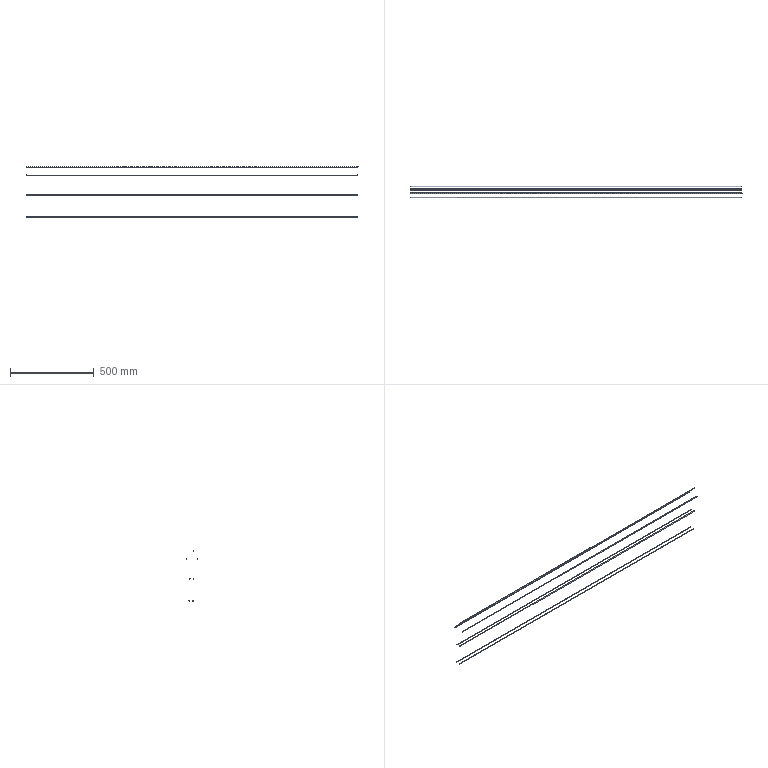Part | SolidWorks | features BaseBody 7 | 7 solids | 28 faces | box 1977 x 68.151 x 299.907 mm | volume 173588 mm3 | cylinder 14 | plane 14 | commonest cylinder face diameters 4 x14
STEP:
#1=CARTESIAN_POINT('',(-25.106,43.452,97.628));
#2=VERTEX_POINT('',#1);
#3=CARTESIAN_POINT('',(-25.106,39.452,97.628));
#4=VERTEX_POINT('',#3);
#5=CARTESIAN_POINT('',(-25.106,43.452,97.628));
#6=CARTESIAN_POINT('',(-24.91,43.452,101.628));
#7=CARTESIAN_POINT('',(-24.91,39.452,101.628));
#8=CARTESIAN_POINT('',(-25.106,39.452,97.628));
#9=(BOUNDED_CURVE()B_SPLINE_CURVE(3,(#5,#6,#7,#8),.UNSPECIFIED.,.F.,.F.)B_SPLINE_CURVE_WITH_KNOTS((4,4),(1.571,4.712),.UNSPECIFIED.)CURVE()GEOMETRIC_REPRESENTATION_ITEM()RATIONAL_B_SPLINE_CURVE((1.,0.3333,0.3333,1.))REPRESENTATION_ITEM(''));
#10=EDGE_CURVE('',#2,#4,#9,.T.);
#11=ORIENTED_EDGE('',*,*,#10,.F.);
#12=CARTESIAN_POINT('',(-2000.,43.452,97.628));
#13=VERTEX_POINT('',#12);
#14=CARTESIAN_POINT('',(-13.158,43.452,97.628));
#15=DIRECTION('',(-1.,0.,0.));
#16=VECTOR('',#15,1000.);
#17=LINE('',#14,#16);
#18=EDGE_CURVE('',#2,#13,#17,.T.);
#19=ORIENTED_EDGE('',*,*,#18,.T.);
#20=CARTESIAN_POINT('',(-2000.,39.452,97.628));
#21=VERTEX_POINT('',#20);
#22=CARTESIAN_POINT('',(-2000.,41.452,97.628));
#23=DIRECTION('',(-1.,0.,0.));
#24=DIRECTION('',(0.,-1.,0.));
#25=AXIS2_PLACEMENT_3D('',#22,#23,#24);
#26=CIRCLE('',#25,2.);
#27=EDGE_CURVE('',#21,#13,#26,.T.);
#28=ORIENTED_EDGE('',*,*,#27,.F.);
#29=CARTESIAN_POINT('',(-13.158,39.452,97.628));
#30=DIRECTION('',(-1.,0.,0.));
#31=VECTOR('',#30,1000.);
#32=LINE('',#29,#31);
#33=EDGE_CURVE('',#4,#21,#32,.T.);
#34=ORIENTED_EDGE('',*,*,#33,.F.);
#35=EDGE_LOOP('',(#11,#19,#28,#34));
#36=FACE_OUTER_BOUND('',#35,.T.);
#37=CARTESIAN_POINT('',(-13.158,41.452,97.628));
#38=DIRECTION('',(-1.,0.,0.));
#39=DIRECTION('',(0.,-1.,0.));
#40=AXIS2_PLACEMENT_3D('',#37,#38,#39);
#41=CYLINDRICAL_SURFACE('',#40,2.);
#42=ADVANCED_FACE('',(#36),#41,.T.);
#43=ORIENTED_EDGE('',*,*,#18,.F.);
#44=CARTESIAN_POINT('',(-25.106,39.452,97.628));
#45=CARTESIAN_POINT('',(-25.302,39.452,93.628));
#46=CARTESIAN_POINT('',(-25.302,43.452,93.628));
#47=CARTESIAN_POINT('',(-25.106,43.452,97.628));
#48=(BOUNDED_CURVE()B_SPLINE_CURVE(3,(#44,#45,#46,#47),.UNSPECIFIED.,.F.,.F.)B_SPLINE_CURVE_WITH_KNOTS((4,4),(4.712,7.854),.UNSPECIFIED.)CURVE()GEOMETRIC_REPRESENTATION_ITEM()RATIONAL_B_SPLINE_CURVE((1.,0.3333,0.3333,1.))REPRESENTATION_ITEM(''));
#49=EDGE_CURVE('',#4,#2,#48,.T.);
#50=ORIENTED_EDGE('',*,*,#49,.F.);
#51=ORIENTED_EDGE('',*,*,#33,.T.);
#52=CARTESIAN_POINT('',(-2000.,41.452,97.628));
#53=DIRECTION('',(-1.,0.,0.));
#54=DIRECTION('',(0.,-1.,0.));
#55=AXIS2_PLACEMENT_3D('',#52,#53,#54);
#56=CIRCLE('',#55,2.);
#57=EDGE_CURVE('',#13,#21,#56,.T.);
#58=ORIENTED_EDGE('',*,*,#57,.F.);
#59=EDGE_LOOP('',(#43,#50,#51,#58));
#60=FACE_OUTER_BOUND('',#59,.T.);
#61=CARTESIAN_POINT('',(-13.158,41.452,97.628));
#62=DIRECTION('',(-1.,0.,0.));
#63=DIRECTION('',(0.,-1.,0.));
#64=AXIS2_PLACEMENT_3D('',#61,#62,#63);
#65=CYLINDRICAL_SURFACE('',#64,2.);
#66=ADVANCED_FACE('',(#60),#65,.T.);
#67=ORIENTED_EDGE('',*,*,#49,.T.);
#68=ORIENTED_EDGE('',*,*,#10,.T.);
#69=EDGE_LOOP('',(#67,#68));
#70=FACE_OUTER_BOUND('',#69,.T.);
#71=CARTESIAN_POINT('',(-25.205,39.428,95.604));
#72=DIRECTION('',(-0.9988,0.,0.04903));
#73=DIRECTION('',(0.04903,0.,0.9988));
#74=AXIS2_PLACEMENT_3D('',#71,#72,#73);
#75=PLANE('',#74);
#76=ADVANCED_FACE('',(#70),#75,.F.);
#77=ORIENTED_EDGE('',*,*,#27,.T.);
#78=ORIENTED_EDGE('',*,*,#57,.T.);
#79=EDGE_LOOP('',(#77,#78));
#80=FACE_OUTER_BOUND('',#79,.T.);
#81=CARTESIAN_POINT('',(-2000.,39.428,99.652));
#82=DIRECTION('',(1.,0.,0.));
#83=DIRECTION('',(0.,0.,-1.));
#84=AXIS2_PLACEMENT_3D('',#81,#82,#83);
#85=PLANE('',#84);
#86=ADVANCED_FACE('',(#80),#85,.F.);
#87=CLOSED_SHELL('',(#42,#66,#76,#86));
#88=MANIFOLD_SOLID_BREP('',#87);
#89=CARTESIAN_POINT('',(-25.106,-20.7,97.628));
#90=VERTEX_POINT('',#89);
#91=CARTESIAN_POINT('',(-25.106,-24.7,97.628));
#92=VERTEX_POINT('',#91);
#93=CARTESIAN_POINT('',(-25.106,-20.7,97.628));
#94=CARTESIAN_POINT('',(-24.91,-20.7,101.628));
#95=CARTESIAN_POINT('',(-24.91,-24.7,101.628));
#96=CARTESIAN_POINT('',(-25.106,-24.7,97.628));
#97=(BOUNDED_CURVE()B_SPLINE_CURVE(3,(#93,#94,#95,#96),.UNSPECIFIED.,.F.,.F.)B_SPLINE_CURVE_WITH_KNOTS((4,4),(1.571,4.712),.UNSPECIFIED.)CURVE()GEOMETRIC_REPRESENTATION_ITEM()RATIONAL_B_SPLINE_CURVE((1.,0.3333,0.3333,1.))REPRESENTATION_ITEM(''));
#98=EDGE_CURVE('',#90,#92,#97,.T.);
#99=ORIENTED_EDGE('',*,*,#98,.F.);
#100=CARTESIAN_POINT('',(-2000.,-20.7,97.628));
#101=VERTEX_POINT('',#100);
#102=CARTESIAN_POINT('',(-13.158,-20.7,97.628));
#103=DIRECTION('',(-1.,0.,0.));
#104=VECTOR('',#103,1000.);
#105=LINE('',#102,#104);
#106=EDGE_CURVE('',#90,#101,#105,.T.);
#107=ORIENTED_EDGE('',*,*,#106,.T.);
#108=CARTESIAN_POINT('',(-2000.,-24.7,97.628));
#109=VERTEX_POINT('',#108);
#110=CARTESIAN_POINT('',(-2000.,-22.7,97.628));
#111=DIRECTION('',(-1.,0.,0.));
#112=DIRECTION('',(0.,-1.,0.));
#113=AXIS2_PLACEMENT_3D('',#110,#111,#112);
#114=CIRCLE('',#113,2.);
#115=EDGE_CURVE('',#109,#101,#114,.T.);
#116=ORIENTED_EDGE('',*,*,#115,.F.);
#117=CARTESIAN_POINT('',(-13.158,-24.7,97.628));
#118=DIRECTION('',(-1.,0.,0.));
#119=VECTOR('',#118,1000.);
#120=LINE('',#117,#119);
#121=EDGE_CURVE('',#92,#109,#120,.T.);
#122=ORIENTED_EDGE('',*,*,#121,.F.);
#123=EDGE_LOOP('',(#99,#107,#116,#122));
#124=FACE_OUTER_BOUND('',#123,.T.);
#125=CARTESIAN_POINT('',(-13.158,-22.7,97.628));
#126=DIRECTION('',(-1.,0.,0.));
#127=DIRECTION('',(0.,-1.,0.));
#128=AXIS2_PLACEMENT_3D('',#125,#126,#127);
#129=CYLINDRICAL_SURFACE('',#128,2.);
#130=ADVANCED_FACE('',(#124),#129,.T.);
#131=ORIENTED_EDGE('',*,*,#106,.F.);
#132=CARTESIAN_POINT('',(-25.106,-24.7,97.628));
#133=CARTESIAN_POINT('',(-25.302,-24.7,93.628));
#134=CARTESIAN_POINT('',(-25.302,-20.7,93.628));
#135=CARTESIAN_POINT('',(-25.106,-20.7,97.628));
#136=(BOUNDED_CURVE()B_SPLINE_CURVE(3,(#132,#133,#134,#135),.UNSPECIFIED.,.F.,.F.)B_SPLINE_CURVE_WITH_KNOTS((4,4),(4.712,7.854),.UNSPECIFIED.)CURVE()GEOMETRIC_REPRESENTATION_ITEM()RATIONAL_B_SPLINE_CURVE((1.,0.3333,0.3333,1.))REPRESENTATION_ITEM(''));
#137=EDGE_CURVE('',#92,#90,#136,.T.);
#138=ORIENTED_EDGE('',*,*,#137,.F.);
#139=ORIENTED_EDGE('',*,*,#121,.T.);
#140=CARTESIAN_POINT('',(-2000.,-22.7,97.628));
#141=DIRECTION('',(-1.,0.,0.));
#142=DIRECTION('',(0.,-1.,0.));
#143=AXIS2_PLACEMENT_3D('',#140,#141,#142);
#144=CIRCLE('',#143,2.);
#145=EDGE_CURVE('',#101,#109,#144,.T.);
#146=ORIENTED_EDGE('',*,*,#145,.F.);
#147=EDGE_LOOP('',(#131,#138,#139,#146));
#148=FACE_OUTER_BOUND('',#147,.T.);
#149=CARTESIAN_POINT('',(-13.158,-22.7,97.628));
#150=DIRECTION('',(-1.,0.,0.));
#151=DIRECTION('',(0.,-1.,0.));
#152=AXIS2_PLACEMENT_3D('',#149,#150,#151);
#153=CYLINDRICAL_SURFACE('',#152,2.);
#154=ADVANCED_FACE('',(#148),#153,.T.);
#155=ORIENTED_EDGE('',*,*,#137,.T.);
#156=ORIENTED_EDGE('',*,*,#98,.T.);
#157=EDGE_LOOP('',(#155,#156));
#158=FACE_OUTER_BOUND('',#157,.T.);
#159=CARTESIAN_POINT('',(-25.205,-24.724,95.604));
#160=DIRECTION('',(-0.9988,0.,0.04903));
#161=DIRECTION('',(0.04903,0.,0.9988));
#162=AXIS2_PLACEMENT_3D('',#159,#160,#161);
#163=PLANE('',#162);
#164=ADVANCED_FACE('',(#158),#163,.F.);
#165=ORIENTED_EDGE('',*,*,#115,.T.);
#166=ORIENTED_EDGE('',*,*,#145,.T.);
#167=EDGE_LOOP('',(#165,#166));
#168=FACE_OUTER_BOUND('',#167,.T.);
#169=CARTESIAN_POINT('',(-2000.,-24.724,99.652));
#170=DIRECTION('',(1.,0.,0.));
#171=DIRECTION('',(0.,0.,-1.));
#172=AXIS2_PLACEMENT_3D('',#169,#170,#171);
#173=PLANE('',#172);
#174=ADVANCED_FACE('',(#168),#173,.F.);
#175=CLOSED_SHELL('',(#130,#154,#164,#174));
#176=MANIFOLD_SOLID_BREP('',#175);
#177=CARTESIAN_POINT('',(-28.322,27.021,-151.964));
#178=VERTEX_POINT('',#177);
#179=CARTESIAN_POINT('',(-28.322,27.021,-147.964));
#180=VERTEX_POINT('',#179);
#181=CARTESIAN_POINT('',(-28.322,27.021,-149.964));
#182=DIRECTION('',(1.,0.,0.));
#183=DIRECTION('',(0.,0.,1.));
#184=AXIS2_PLACEMENT_3D('',#181,#182,#183);
#185=CIRCLE('',#184,2.);
#186=EDGE_CURVE('',#178,#180,#185,.T.);
#187=ORIENTED_EDGE('',*,*,#186,.F.);
#188=CARTESIAN_POINT('',(-2000.,27.021,-151.964));
#189=VERTEX_POINT('',#188);
#190=CARTESIAN_POINT('',(-28.322,27.021,-151.964));
#191=DIRECTION('',(-1.,0.,0.));
#192=VECTOR('',#191,1000.);
#193=LINE('',#190,#192);
#194=EDGE_CURVE('',#178,#189,#193,.T.);
#195=ORIENTED_EDGE('',*,*,#194,.T.);
#196=CARTESIAN_POINT('',(-2000.,27.021,-147.964));
#197=VERTEX_POINT('',#196);
#198=CARTESIAN_POINT('',(-2000.,27.021,-149.964));
#199=DIRECTION('',(-1.,0.,0.));
#200=DIRECTION('',(0.,0.,1.));
#201=AXIS2_PLACEMENT_3D('',#198,#199,#200);
#202=CIRCLE('',#201,2.);
#203=EDGE_CURVE('',#197,#189,#202,.T.);
#204=ORIENTED_EDGE('',*,*,#203,.F.);
#205=CARTESIAN_POINT('',(-28.322,27.021,-147.964));
#206=DIRECTION('',(-1.,0.,0.));
#207=VECTOR('',#206,1000.);
#208=LINE('',#205,#207);
#209=EDGE_CURVE('',#180,#197,#208,.T.);
#210=ORIENTED_EDGE('',*,*,#209,.F.);
#211=EDGE_LOOP('',(#187,#195,#204,#210));
#212=FACE_OUTER_BOUND('',#211,.T.);
#213=CARTESIAN_POINT('',(-28.322,27.021,-149.964));
#214=DIRECTION('',(-1.,0.,0.));
#215=DIRECTION('',(0.,0.,1.));
#216=AXIS2_PLACEMENT_3D('',#213,#214,#215);
#217=CYLINDRICAL_SURFACE('',#216,2.);
#218=ADVANCED_FACE('',(#212),#217,.T.);
#219=ORIENTED_EDGE('',*,*,#194,.F.);
#220=CARTESIAN_POINT('',(-28.322,27.021,-149.964));
#221=DIRECTION('',(1.,0.,0.));
#222=DIRECTION('',(0.,0.,1.));
#223=AXIS2_PLACEMENT_3D('',#220,#221,#222);
#224=CIRCLE('',#223,2.);
#225=EDGE_CURVE('',#180,#178,#224,.T.);
#226=ORIENTED_EDGE('',*,*,#225,.F.);
#227=ORIENTED_EDGE('',*,*,#209,.T.);
#228=CARTESIAN_POINT('',(-2000.,27.021,-149.964));
#229=DIRECTION('',(-1.,0.,0.));
#230=DIRECTION('',(0.,0.,1.));
#231=AXIS2_PLACEMENT_3D('',#228,#229,#230);
#232=CIRCLE('',#231,2.);
#233=EDGE_CURVE('',#189,#197,#232,.T.);
#234=ORIENTED_EDGE('',*,*,#233,.F.);
#235=EDGE_LOOP('',(#219,#226,#227,#234));
#236=FACE_OUTER_BOUND('',#235,.T.);
#237=CARTESIAN_POINT('',(-28.322,27.021,-149.964));
#238=DIRECTION('',(-1.,0.,0.));
#239=DIRECTION('',(0.,0.,1.));
#240=AXIS2_PLACEMENT_3D('',#237,#238,#239);
#241=CYLINDRICAL_SURFACE('',#240,2.);
#242=ADVANCED_FACE('',(#236),#241,.T.);
#243=ORIENTED_EDGE('',*,*,#225,.T.);
#244=ORIENTED_EDGE('',*,*,#186,.T.);
#245=EDGE_LOOP('',(#243,#244));
#246=FACE_OUTER_BOUND('',#245,.T.);
#247=CARTESIAN_POINT('',(-28.322,24.997,-151.988));
#248=DIRECTION('',(-1.,0.,0.));
#249=DIRECTION('',(0.,0.,1.));
#250=AXIS2_PLACEMENT_3D('',#247,#248,#249);
#251=PLANE('',#250);
#252=ADVANCED_FACE('',(#246),#251,.F.);
#253=ORIENTED_EDGE('',*,*,#203,.T.);
#254=ORIENTED_EDGE('',*,*,#233,.T.);
#255=EDGE_LOOP('',(#253,#254));
#256=FACE_OUTER_BOUND('',#255,.T.);
#257=CARTESIAN_POINT('',(-2000.,24.997,-147.94));
#258=DIRECTION('',(1.,0.,0.));
#259=DIRECTION('',(0.,0.,-1.));
#260=AXIS2_PLACEMENT_3D('',#257,#258,#259);
#261=PLANE('',#260);
#262=ADVANCED_FACE('',(#256),#261,.F.);
#263=CLOSED_SHELL('',(#218,#242,#252,#262));
#264=MANIFOLD_SOLID_BREP('',#263);
#265=CARTESIAN_POINT('',(-28.322,3.953,-152.971));
#266=VERTEX_POINT('',#265);
#267=CARTESIAN_POINT('',(-28.322,3.953,-148.971));
#268=VERTEX_POINT('',#267);
#269=CARTESIAN_POINT('',(-28.322,3.953,-150.971));
#270=DIRECTION('',(1.,0.,0.));
#271=DIRECTION('',(0.,0.,1.));
#272=AXIS2_PLACEMENT_3D('',#269,#270,#271);
#273=CIRCLE('',#272,2.);
#274=EDGE_CURVE('',#266,#268,#273,.T.);
#275=ORIENTED_EDGE('',*,*,#274,.F.);
#276=CARTESIAN_POINT('',(-2000.,3.953,-152.971));
#277=VERTEX_POINT('',#276);
#278=CARTESIAN_POINT('',(-28.322,3.953,-152.971));
#279=DIRECTION('',(-1.,0.,0.));
#280=VECTOR('',#279,1000.);
#281=LINE('',#278,#280);
#282=EDGE_CURVE('',#266,#277,#281,.T.);
#283=ORIENTED_EDGE('',*,*,#282,.T.);
#284=CARTESIAN_POINT('',(-2000.,3.953,-148.971));
#285=VERTEX_POINT('',#284);
#286=CARTESIAN_POINT('',(-2000.,3.953,-150.971));
#287=DIRECTION('',(-1.,0.,0.));
#288=DIRECTION('',(0.,0.,1.));
#289=AXIS2_PLACEMENT_3D('',#286,#287,#288);
#290=CIRCLE('',#289,2.);
#291=EDGE_CURVE('',#285,#277,#290,.T.);
#292=ORIENTED_EDGE('',*,*,#291,.F.);
#293=CARTESIAN_POINT('',(-28.322,3.953,-148.971));
#294=DIRECTION('',(-1.,0.,0.));
#295=VECTOR('',#294,1000.);
#296=LINE('',#293,#295);
#297=EDGE_CURVE('',#268,#285,#296,.T.);
#298=ORIENTED_EDGE('',*,*,#297,.F.);
#299=EDGE_LOOP('',(#275,#283,#292,#298));
#300=FACE_OUTER_BOUND('',#299,.T.);
#301=CARTESIAN_POINT('',(-28.322,3.953,-150.971));
#302=DIRECTION('',(-1.,0.,0.));
#303=DIRECTION('',(0.,0.,1.));
#304=AXIS2_PLACEMENT_3D('',#301,#302,#303);
#305=CYLINDRICAL_SURFACE('',#304,2.);
#306=ADVANCED_FACE('',(#300),#305,.T.);
#307=ORIENTED_EDGE('',*,*,#282,.F.);
#308=CARTESIAN_POINT('',(-28.322,3.953,-150.971));
#309=DIRECTION('',(1.,0.,0.));
#310=DIRECTION('',(0.,0.,1.));
#311=AXIS2_PLACEMENT_3D('',#308,#309,#310);
#312=CIRCLE('',#311,2.);
#313=EDGE_CURVE('',#268,#266,#312,.T.);
#314=ORIENTED_EDGE('',*,*,#313,.F.);
#315=ORIENTED_EDGE('',*,*,#297,.T.);
#316=CARTESIAN_POINT('',(-2000.,3.953,-150.971));
#317=DIRECTION('',(-1.,0.,0.));
#318=DIRECTION('',(0.,0.,1.));
#319=AXIS2_PLACEMENT_3D('',#316,#317,#318);
#320=CIRCLE('',#319,2.);
#321=EDGE_CURVE('',#277,#285,#320,.T.);
#322=ORIENTED_EDGE('',*,*,#321,.F.);
#323=EDGE_LOOP('',(#307,#314,#315,#322));
#324=FACE_OUTER_BOUND('',#323,.T.);
#325=CARTESIAN_POINT('',(-28.322,3.953,-150.971));
#326=DIRECTION('',(-1.,0.,0.));
#327=DIRECTION('',(0.,0.,1.));
#328=AXIS2_PLACEMENT_3D('',#325,#326,#327);
#329=CYLINDRICAL_SURFACE('',#328,2.);
#330=ADVANCED_FACE('',(#324),#329,.T.);
#331=ORIENTED_EDGE('',*,*,#313,.T.);
#332=ORIENTED_EDGE('',*,*,#274,.T.);
#333=EDGE_LOOP('',(#331,#332));
#334=FACE_OUTER_BOUND('',#333,.T.);
#335=CARTESIAN_POINT('',(-28.322,1.929,-152.995));
#336=DIRECTION('',(-1.,0.,0.));
#337=DIRECTION('',(0.,0.,1.));
#338=AXIS2_PLACEMENT_3D('',#335,#336,#337);
#339=PLANE('',#338);
#340=ADVANCED_FACE('',(#334),#339,.F.);
#341=ORIENTED_EDGE('',*,*,#291,.T.);
#342=ORIENTED_EDGE('',*,*,#321,.T.);
#343=EDGE_LOOP('',(#341,#342));
#344=FACE_OUTER_BOUND('',#343,.T.);
#345=CARTESIAN_POINT('',(-2000.,1.929,-148.947));
#346=DIRECTION('',(1.,0.,0.));
#347=DIRECTION('',(0.,0.,-1.));
#348=AXIS2_PLACEMENT_3D('',#345,#346,#347);
#349=PLANE('',#348);
#350=ADVANCED_FACE('',(#344),#349,.F.);
#351=CLOSED_SHELL('',(#306,#330,#340,#350));
#352=MANIFOLD_SOLID_BREP('',#351);
#353=CARTESIAN_POINT('',(-22.882,1.206,142.936));
#354=VERTEX_POINT('',#353);
#355=CARTESIAN_POINT('',(-22.686,1.206,146.936));
#356=VERTEX_POINT('',#355);
#357=CARTESIAN_POINT('',(-22.882,1.206,142.936));
#358=CARTESIAN_POINT('',(-22.882,5.206,142.936));
#359=CARTESIAN_POINT('',(-22.686,5.206,146.936));
#360=CARTESIAN_POINT('',(-22.686,1.206,146.936));
#361=(BOUNDED_CURVE()B_SPLINE_CURVE(3,(#357,#358,#359,#360),.UNSPECIFIED.,.F.,.F.)B_SPLINE_CURVE_WITH_KNOTS((4,4),(0.,3.142),.UNSPECIFIED.)CURVE()GEOMETRIC_REPRESENTATION_ITEM()RATIONAL_B_SPLINE_CURVE((1.,0.3333,0.3333,1.))REPRESENTATION_ITEM(''));
#362=EDGE_CURVE('',#354,#356,#361,.T.);
#363=ORIENTED_EDGE('',*,*,#362,.F.);
#364=CARTESIAN_POINT('',(-2000.,1.206,142.936));
#365=VERTEX_POINT('',#364);
#366=CARTESIAN_POINT('',(-10.822,1.206,142.936));
#367=DIRECTION('',(-1.,0.,0.));
#368=VECTOR('',#367,1000.);
#369=LINE('',#366,#368);
#370=EDGE_CURVE('',#354,#365,#369,.T.);
#371=ORIENTED_EDGE('',*,*,#370,.T.);
#372=CARTESIAN_POINT('',(-2000.,1.206,146.936));
#373=VERTEX_POINT('',#372);
#374=CARTESIAN_POINT('',(-2000.,1.206,144.936));
#375=DIRECTION('',(-1.,0.,0.));
#376=DIRECTION('',(0.,0.,1.));
#377=AXIS2_PLACEMENT_3D('',#374,#375,#376);
#378=CIRCLE('',#377,2.);
#379=EDGE_CURVE('',#373,#365,#378,.T.);
#380=ORIENTED_EDGE('',*,*,#379,.F.);
#381=CARTESIAN_POINT('',(-10.822,1.206,146.936));
#382=DIRECTION('',(-1.,0.,0.));
#383=VECTOR('',#382,1000.);
#384=LINE('',#381,#383);
#385=EDGE_CURVE('',#356,#373,#384,.T.);
#386=ORIENTED_EDGE('',*,*,#385,.F.);
#387=EDGE_LOOP('',(#363,#371,#380,#386));
#388=FACE_OUTER_BOUND('',#387,.T.);
#389=CARTESIAN_POINT('',(-10.822,1.206,144.936));
#390=DIRECTION('',(-1.,0.,0.));
#391=DIRECTION('',(0.,0.,1.));
#392=AXIS2_PLACEMENT_3D('',#389,#390,#391);
#393=CYLINDRICAL_SURFACE('',#392,2.);
#394=ADVANCED_FACE('',(#388),#393,.T.);
#395=ORIENTED_EDGE('',*,*,#370,.F.);
#396=CARTESIAN_POINT('',(-22.686,1.206,146.936));
#397=CARTESIAN_POINT('',(-22.686,-2.794,146.936));
#398=CARTESIAN_POINT('',(-22.882,-2.794,142.936));
#399=CARTESIAN_POINT('',(-22.882,1.206,142.936));
#400=(BOUNDED_CURVE()B_SPLINE_CURVE(3,(#396,#397,#398,#399),.UNSPECIFIED.,.F.,.F.)B_SPLINE_CURVE_WITH_KNOTS((4,4),(3.142,6.283),.UNSPECIFIED.)CURVE()GEOMETRIC_REPRESENTATION_ITEM()RATIONAL_B_SPLINE_CURVE((1.,0.3333,0.3333,1.))REPRESENTATION_ITEM(''));
#401=EDGE_CURVE('',#356,#354,#400,.T.);
#402=ORIENTED_EDGE('',*,*,#401,.F.);
#403=ORIENTED_EDGE('',*,*,#385,.T.);
#404=CARTESIAN_POINT('',(-2000.,1.206,144.936));
#405=DIRECTION('',(-1.,0.,0.));
#406=DIRECTION('',(0.,0.,1.));
#407=AXIS2_PLACEMENT_3D('',#404,#405,#406);
#408=CIRCLE('',#407,2.);
#409=EDGE_CURVE('',#365,#373,#408,.T.);
#410=ORIENTED_EDGE('',*,*,#409,.F.);
#411=EDGE_LOOP('',(#395,#402,#403,#410));
#412=FACE_OUTER_BOUND('',#411,.T.);
#413=CARTESIAN_POINT('',(-10.822,1.206,144.936));
#414=DIRECTION('',(-1.,0.,0.));
#415=DIRECTION('',(0.,0.,1.));
#416=AXIS2_PLACEMENT_3D('',#413,#414,#415);
#417=CYLINDRICAL_SURFACE('',#416,2.);
#418=ADVANCED_FACE('',(#412),#417,.T.);
#419=ORIENTED_EDGE('',*,*,#401,.T.);
#420=ORIENTED_EDGE('',*,*,#362,.T.);
#421=EDGE_LOOP('',(#419,#420));
#422=FACE_OUTER_BOUND('',#421,.T.);
#423=CARTESIAN_POINT('',(-22.883,-0.8176,142.912));
#424=DIRECTION('',(-0.9988,0.,0.04903));
#425=DIRECTION('',(0.04903,0.,0.9988));
#426=AXIS2_PLACEMENT_3D('',#423,#424,#425);
#427=PLANE('',#426);
#428=ADVANCED_FACE('',(#422),#427,.F.);
#429=ORIENTED_EDGE('',*,*,#379,.T.);
#430=ORIENTED_EDGE('',*,*,#409,.T.);
#431=EDGE_LOOP('',(#429,#430));
#432=FACE_OUTER_BOUND('',#431,.T.);
#433=CARTESIAN_POINT('',(-2000.,-0.8176,146.96));
#434=DIRECTION('',(1.,0.,0.));
#435=DIRECTION('',(0.,0.,-1.));
#436=AXIS2_PLACEMENT_3D('',#433,#434,#435);
#437=PLANE('',#436);
#438=ADVANCED_FACE('',(#432),#437,.F.);
#439=CLOSED_SHELL('',(#394,#418,#428,#438));
#440=MANIFOLD_SOLID_BREP('',#439);
#441=CARTESIAN_POINT('',(-28.322,0.5236,-21.996));
#442=VERTEX_POINT('',#441);
#443=CARTESIAN_POINT('',(-28.322,0.5236,-17.996));
#444=VERTEX_POINT('',#443);
#445=CARTESIAN_POINT('',(-28.322,0.5236,-19.996));
#446=DIRECTION('',(1.,0.,0.));
#447=DIRECTION('',(0.,0.,1.));
#448=AXIS2_PLACEMENT_3D('',#445,#446,#447);
#449=CIRCLE('',#448,2.);
#450=EDGE_CURVE('',#442,#444,#449,.T.);
#451=ORIENTED_EDGE('',*,*,#450,.F.);
#452=CARTESIAN_POINT('',(-2000.,0.5236,-21.996));
#453=VERTEX_POINT('',#452);
#454=CARTESIAN_POINT('',(-28.322,0.5236,-21.996));
#455=DIRECTION('',(-1.,0.,0.));
#456=VECTOR('',#455,1000.);
#457=LINE('',#454,#456);
#458=EDGE_CURVE('',#442,#453,#457,.T.);
#459=ORIENTED_EDGE('',*,*,#458,.T.);
#460=CARTESIAN_POINT('',(-2000.,0.5236,-17.996));
#461=VERTEX_POINT('',#460);
#462=CARTESIAN_POINT('',(-2000.,0.5236,-19.996));
#463=DIRECTION('',(-1.,0.,0.));
#464=DIRECTION('',(0.,0.,1.));
#465=AXIS2_PLACEMENT_3D('',#462,#463,#464);
#466=CIRCLE('',#465,2.);
#467=EDGE_CURVE('',#461,#453,#466,.T.);
#468=ORIENTED_EDGE('',*,*,#467,.F.);
#469=CARTESIAN_POINT('',(-28.322,0.5236,-17.996));
#470=DIRECTION('',(-1.,0.,0.));
#471=VECTOR('',#470,1000.);
#472=LINE('',#469,#471);
#473=EDGE_CURVE('',#444,#461,#472,.T.);
#474=ORIENTED_EDGE('',*,*,#473,.F.);
#475=EDGE_LOOP('',(#451,#459,#468,#474));
#476=FACE_OUTER_BOUND('',#475,.T.);
#477=CARTESIAN_POINT('',(-28.322,0.5236,-19.996));
#478=DIRECTION('',(-1.,0.,0.));
#479=DIRECTION('',(0.,0.,1.));
#480=AXIS2_PLACEMENT_3D('',#477,#478,#479);
#481=CYLINDRICAL_SURFACE('',#480,2.);
#482=ADVANCED_FACE('',(#476),#481,.T.);
#483=ORIENTED_EDGE('',*,*,#458,.F.);
#484=CARTESIAN_POINT('',(-28.322,0.5236,-19.996));
#485=DIRECTION('',(1.,0.,0.));
#486=DIRECTION('',(0.,0.,1.));
#487=AXIS2_PLACEMENT_3D('',#484,#485,#486);
#488=CIRCLE('',#487,2.);
#489=EDGE_CURVE('',#444,#442,#488,.T.);
#490=ORIENTED_EDGE('',*,*,#489,.F.);
#491=ORIENTED_EDGE('',*,*,#473,.T.);
#492=CARTESIAN_POINT('',(-2000.,0.5236,-19.996));
#493=DIRECTION('',(-1.,0.,0.));
#494=DIRECTION('',(0.,0.,1.));
#495=AXIS2_PLACEMENT_3D('',#492,#493,#494);
#496=CIRCLE('',#495,2.);
#497=EDGE_CURVE('',#453,#461,#496,.T.);
#498=ORIENTED_EDGE('',*,*,#497,.F.);
#499=EDGE_LOOP('',(#483,#490,#491,#498));
#500=FACE_OUTER_BOUND('',#499,.T.);
#501=CARTESIAN_POINT('',(-28.322,0.5236,-19.996));
#502=DIRECTION('',(-1.,0.,0.));
#503=DIRECTION('',(0.,0.,1.));
#504=AXIS2_PLACEMENT_3D('',#501,#502,#503);
#505=CYLINDRICAL_SURFACE('',#504,2.);
#506=ADVANCED_FACE('',(#500),#505,.T.);
#507=ORIENTED_EDGE('',*,*,#489,.T.);
#508=ORIENTED_EDGE('',*,*,#450,.T.);
#509=EDGE_LOOP('',(#507,#508));
#510=FACE_OUTER_BOUND('',#509,.T.);
#511=CARTESIAN_POINT('',(-28.322,-1.5,-22.02));
#512=DIRECTION('',(-1.,0.,0.));
#513=DIRECTION('',(0.,0.,1.));
#514=AXIS2_PLACEMENT_3D('',#511,#512,#513);
#515=PLANE('',#514);
#516=ADVANCED_FACE('',(#510),#515,.F.);
#517=ORIENTED_EDGE('',*,*,#467,.T.);
#518=ORIENTED_EDGE('',*,*,#497,.T.);
#519=EDGE_LOOP('',(#517,#518));
#520=FACE_OUTER_BOUND('',#519,.T.);
#521=CARTESIAN_POINT('',(-2000.,-1.5,-17.972));
#522=DIRECTION('',(1.,0.,0.));
#523=DIRECTION('',(0.,0.,-1.));
#524=AXIS2_PLACEMENT_3D('',#521,#522,#523);
#525=PLANE('',#524);
#526=ADVANCED_FACE('',(#520),#525,.F.);
#527=CLOSED_SHELL('',(#482,#506,#516,#526));
#528=MANIFOLD_SOLID_BREP('',#527);
#529=CARTESIAN_POINT('',(-28.322,22.506,-21.036));
#530=VERTEX_POINT('',#529);
#531=CARTESIAN_POINT('',(-28.322,22.506,-17.036));
#532=VERTEX_POINT('',#531);
#533=CARTESIAN_POINT('',(-28.322,22.506,-19.036));
#534=DIRECTION('',(1.,0.,0.));
#535=DIRECTION('',(0.,0.,1.));
#536=AXIS2_PLACEMENT_3D('',#533,#534,#535);
#537=CIRCLE('',#536,2.);
#538=EDGE_CURVE('',#530,#532,#537,.T.);
#539=ORIENTED_EDGE('',*,*,#538,.F.);
#540=CARTESIAN_POINT('',(-2000.,22.506,-21.036));
#541=VERTEX_POINT('',#540);
#542=CARTESIAN_POINT('',(-28.322,22.506,-21.036));
#543=DIRECTION('',(-1.,0.,0.));
#544=VECTOR('',#543,1000.);
#545=LINE('',#542,#544);
#546=EDGE_CURVE('',#530,#541,#545,.T.);
#547=ORIENTED_EDGE('',*,*,#546,.T.);
#548=CARTESIAN_POINT('',(-2000.,22.506,-17.036));
#549=VERTEX_POINT('',#548);
#550=CARTESIAN_POINT('',(-2000.,22.506,-19.036));
#551=DIRECTION('',(-1.,0.,0.));
#552=DIRECTION('',(0.,0.,1.));
#553=AXIS2_PLACEMENT_3D('',#550,#551,#552);
#554=CIRCLE('',#553,2.);
#555=EDGE_CURVE('',#549,#541,#554,.T.);
#556=ORIENTED_EDGE('',*,*,#555,.F.);
#557=CARTESIAN_POINT('',(-28.322,22.506,-17.036));
#558=DIRECTION('',(-1.,0.,0.));
#559=VECTOR('',#558,1000.);
#560=LINE('',#557,#559);
#561=EDGE_CURVE('',#532,#549,#560,.T.);
#562=ORIENTED_EDGE('',*,*,#561,.F.);
#563=EDGE_LOOP('',(#539,#547,#556,#562));
#564=FACE_OUTER_BOUND('',#563,.T.);
#565=CARTESIAN_POINT('',(-28.322,22.506,-19.036));
#566=DIRECTION('',(-1.,0.,0.));
#567=DIRECTION('',(0.,0.,1.));
#568=AXIS2_PLACEMENT_3D('',#565,#566,#567);
#569=CYLINDRICAL_SURFACE('',#568,2.);
#570=ADVANCED_FACE('',(#564),#569,.T.);
#571=ORIENTED_EDGE('',*,*,#546,.F.);
#572=CARTESIAN_POINT('',(-28.322,22.506,-19.036));
#573=DIRECTION('',(1.,0.,0.));
#574=DIRECTION('',(0.,0.,1.));
#575=AXIS2_PLACEMENT_3D('',#572,#573,#574);
#576=CIRCLE('',#575,2.);
#577=EDGE_CURVE('',#532,#530,#576,.T.);
#578=ORIENTED_EDGE('',*,*,#577,.F.);
#579=ORIENTED_EDGE('',*,*,#561,.T.);
#580=CARTESIAN_POINT('',(-2000.,22.506,-19.036));
#581=DIRECTION('',(-1.,0.,0.));
#582=DIRECTION('',(0.,0.,1.));
#583=AXIS2_PLACEMENT_3D('',#580,#581,#582);
#584=CIRCLE('',#583,2.);
#585=EDGE_CURVE('',#541,#549,#584,.T.);
#586=ORIENTED_EDGE('',*,*,#585,.F.);
#587=EDGE_LOOP('',(#571,#578,#579,#586));
#588=FACE_OUTER_BOUND('',#587,.T.);
#589=CARTESIAN_POINT('',(-28.322,22.506,-19.036));
#590=DIRECTION('',(-1.,0.,0.));
#591=DIRECTION('',(0.,0.,1.));
#592=AXIS2_PLACEMENT_3D('',#589,#590,#591);
#593=CYLINDRICAL_SURFACE('',#592,2.);
#594=ADVANCED_FACE('',(#588),#593,.T.);
#595=ORIENTED_EDGE('',*,*,#577,.T.);
#596=ORIENTED_EDGE('',*,*,#538,.T.);
#597=EDGE_LOOP('',(#595,#596));
#598=FACE_OUTER_BOUND('',#597,.T.);
#599=CARTESIAN_POINT('',(-28.322,20.482,-21.06));
#600=DIRECTION('',(-1.,0.,0.));
#601=DIRECTION('',(0.,0.,1.));
#602=AXIS2_PLACEMENT_3D('',#599,#600,#601);
#603=PLANE('',#602);
#604=ADVANCED_FACE('',(#598),#603,.F.);
#605=ORIENTED_EDGE('',*,*,#555,.T.);
#606=ORIENTED_EDGE('',*,*,#585,.T.);
#607=EDGE_LOOP('',(#605,#606));
#608=FACE_OUTER_BOUND('',#607,.T.);
#609=CARTESIAN_POINT('',(-2000.,20.482,-17.012));
#610=DIRECTION('',(1.,0.,0.));
#611=DIRECTION('',(0.,0.,-1.));
#612=AXIS2_PLACEMENT_3D('',#609,#610,#611);
#613=PLANE('',#612);
#614=ADVANCED_FACE('',(#608),#613,.F.);
#615=CLOSED_SHELL('',(#570,#594,#604,#614));
#616=MANIFOLD_SOLID_BREP('',#615);
#617=CARTESIAN_POINT('',(0.,0.,0.));
#618=DIRECTION('',(0.,0.,1.));
#619=DIRECTION('',(1.,0.,0.));
#620=AXIS2_PLACEMENT_3D('',#617,#618,#619);
#621=(LENGTH_UNIT()NAMED_UNIT(*)SI_UNIT(.MILLI.,.METRE.));
#622=UNCERTAINTY_MEASURE_WITH_UNIT(LENGTH_MEASURE(0.00001),#621,'','');
#623=(NAMED_UNIT(*)PLANE_ANGLE_UNIT()SI_UNIT($,.RADIAN.));
#624=(NAMED_UNIT(*)SI_UNIT($,.STERADIAN.)SOLID_ANGLE_UNIT());
#625=(GEOMETRIC_REPRESENTATION_CONTEXT(3)GLOBAL_UNCERTAINTY_ASSIGNED_CONTEXT((#622))GLOBAL_UNIT_ASSIGNED_CONTEXT((#621,#623,#624))REPRESENTATION_CONTEXT('',''));
#626=ADVANCED_BREP_SHAPE_REPRESENTATION('',(#88,#176,#264,#352,#440,#528,#616,#620),#625);